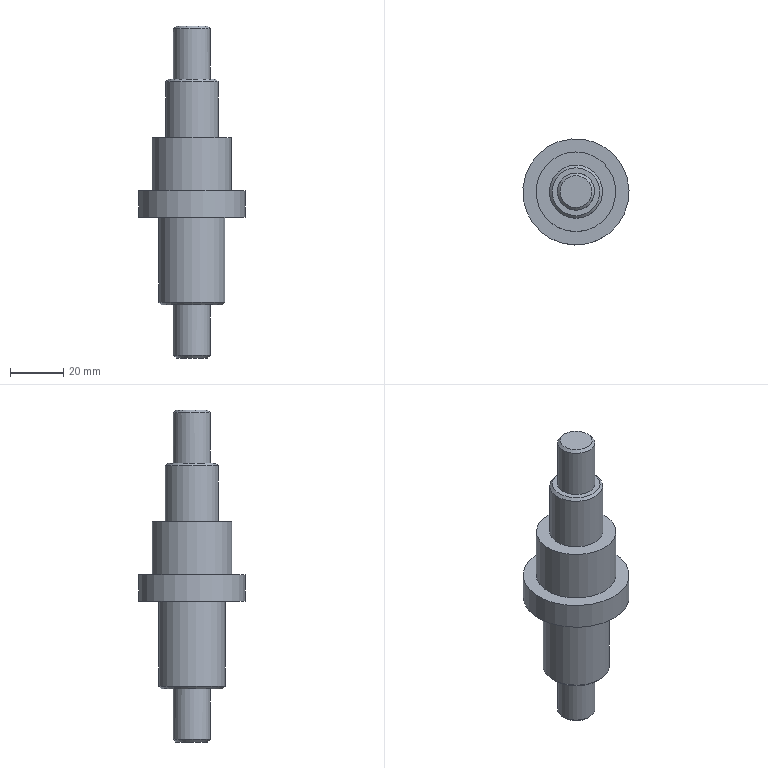Part | STEP file | HL4GZ-1.313.202 (eye-ring mounting shaft) | 1 solid | 17 faces | box 40 x 40 x 125 mm | volume 55861 mm3 | plane 7 | cylinder 6 | cone 4 | commonest cylinder face diameters 14 x2 20 x1 25 x1 30 x1 40 x1
STEP:
#1=CARTESIAN_POINT('',(0.,0.,0.));
#2=DIRECTION('',(0.,0.,1.));
#3=DIRECTION('',(1.,0.,0.));
#4=AXIS2_PLACEMENT_3D('',#1,#2,#3);
#5=CARTESIAN_POINT('',(2574.634,152.537,54.));
#6=VERTEX_POINT('',#5);
#7=CARTESIAN_POINT('',(2570.663,148.04,54.));
#8=DIRECTION('',(0.,0.,-1.));
#9=DIRECTION('',(-0.6618,-0.7497,0.));
#10=AXIS2_PLACEMENT_3D('',#7,#8,#9);
#11=CIRCLE('',#10,6.);
#12=CARTESIAN_POINT('',(2566.03,142.792,54.));
#13=DIRECTION('',(0.,0.,1.));
#14=DIRECTION('',(-0.1489,0.9889,0.));
#15=AXIS2_PLACEMENT_3D('',#12,#13,#14);
#16=PLANE('',#15);
#17=CARTESIAN_POINT('',(0.6428,-0.766));
#18=CARTESIAN_POINT('',(8.604,5.914));
#19=CARTESIAN_POINT('',(10.408,-4.32));
#20=CARTESIAN_POINT('',(12.213,-14.555));
#21=CARTESIAN_POINT('',(2.447,-11.));
#22=CARTESIAN_POINT('',(-7.318,-7.446));
#23=CARTESIAN_POINT('',(0.6428,-0.766));
#24=(BOUNDED_CURVE()B_SPLINE_CURVE(2,(#17,#18,#19,#20,#21,#22,#23),.UNSPECIFIED.,.T.,.F.)B_SPLINE_CURVE_WITH_KNOTS((1,2,2,2,2,1),(-2.094,0.,2.094,4.189,6.283,8.378),.UNSPECIFIED.)CURVE()GEOMETRIC_REPRESENTATION_ITEM()RATIONAL_B_SPLINE_CURVE((1.,0.5,1.,0.5,1.,0.5,1.))REPRESENTATION_ITEM(''));
#25=(GEOMETRIC_REPRESENTATION_CONTEXT(2)PARAMETRIC_REPRESENTATION_CONTEXT()REPRESENTATION_CONTEXT('',''));
#26=DEFINITIONAL_REPRESENTATION('',(#24),#25);
#27=PCURVE('',#16,#26);
#28=CARTESIAN_POINT('',(2570.663,148.04,53.5));
#29=DIRECTION('',(0.,0.,-1.));
#30=DIRECTION('',(-0.6618,-0.7497,0.));
#31=AXIS2_PLACEMENT_3D('',#28,#29,#30);
#32=CONICAL_SURFACE('',#31,6.5,0.7854);
#33=CARTESIAN_POINT('',(0.,-0.5));
#34=DIRECTION('',(1.,0.));
#35=VECTOR('',#34,1.);
#36=LINE('',#33,#35);
#37=(GEOMETRIC_REPRESENTATION_CONTEXT(2)PARAMETRIC_REPRESENTATION_CONTEXT()REPRESENTATION_CONTEXT('',''));
#38=DEFINITIONAL_REPRESENTATION('',(#36),#37);
#39=PCURVE('',#32,#38);
#40=SURFACE_CURVE('',#11,(#27,#39),.PCURVE_S1.);
#41=EDGE_CURVE('',#6,#6,#40,.T.);
#42=ORIENTED_EDGE('',*,*,#41,.F.);
#43=EDGE_LOOP('',(#42));
#44=FACE_BOUND('',#43,.T.);
#45=ADVANCED_FACE('',(#44),#16,.T.);
#46=CARTESIAN_POINT('',(2575.296,153.287,53.));
#47=VERTEX_POINT('',#46);
#48=CARTESIAN_POINT('',(2577.585,149.082,53.));
#49=VERTEX_POINT('',#48);
#50=CARTESIAN_POINT('',(2570.663,148.04,53.));
#51=DIRECTION('',(0.,0.,1.));
#52=DIRECTION('',(-0.6618,-0.7497,0.));
#53=AXIS2_PLACEMENT_3D('',#50,#51,#52);
#54=CIRCLE('',#53,7.);
#55=CARTESIAN_POINT('',(12.566,0.5));
#56=DIRECTION('',(-1.,0.));
#57=VECTOR('',#56,1.);
#58=LINE('',#55,#57);
#59=(GEOMETRIC_REPRESENTATION_CONTEXT(2)PARAMETRIC_REPRESENTATION_CONTEXT()REPRESENTATION_CONTEXT('',''));
#60=DEFINITIONAL_REPRESENTATION('',(#58),#59);
#61=PCURVE('',#32,#60);
#62=CARTESIAN_POINT('',(2570.663,148.04,37.));
#63=DIRECTION('',(0.,0.,-1.));
#64=DIRECTION('',(-0.6618,-0.7497,0.));
#65=AXIS2_PLACEMENT_3D('',#62,#63,#64);
#66=CYLINDRICAL_SURFACE('',#65,7.);
#67=CARTESIAN_POINT('',(12.566,-16.));
#68=DIRECTION('',(-1.,0.));
#69=VECTOR('',#68,1.);
#70=LINE('',#67,#69);
#71=(GEOMETRIC_REPRESENTATION_CONTEXT(2)PARAMETRIC_REPRESENTATION_CONTEXT()REPRESENTATION_CONTEXT('',''));
#72=DEFINITIONAL_REPRESENTATION('',(#70),#71);
#73=PCURVE('',#66,#72);
#74=SURFACE_CURVE('',#54,(#61,#73),.PCURVE_S1.);
#75=EDGE_CURVE('',#47,#49,#74,.T.);
#76=ORIENTED_EDGE('',*,*,#75,.T.);
#77=CARTESIAN_POINT('',(2570.663,148.04,53.));
#78=DIRECTION('',(0.,0.,1.));
#79=DIRECTION('',(-0.6618,-0.7497,0.));
#80=AXIS2_PLACEMENT_3D('',#77,#78,#79);
#81=CIRCLE('',#80,7.);
#82=CARTESIAN_POINT('',(6.283,0.5));
#83=DIRECTION('',(-1.,0.));
#84=VECTOR('',#83,1.);
#85=LINE('',#82,#84);
#86=(GEOMETRIC_REPRESENTATION_CONTEXT(2)PARAMETRIC_REPRESENTATION_CONTEXT()REPRESENTATION_CONTEXT('',''));
#87=DEFINITIONAL_REPRESENTATION('',(#85),#86);
#88=PCURVE('',#32,#87);
#89=CARTESIAN_POINT('',(12.566,-16.));
#90=DIRECTION('',(-1.,0.));
#91=VECTOR('',#90,1.);
#92=LINE('',#89,#91);
#93=(GEOMETRIC_REPRESENTATION_CONTEXT(2)PARAMETRIC_REPRESENTATION_CONTEXT()REPRESENTATION_CONTEXT('',''));
#94=DEFINITIONAL_REPRESENTATION('',(#92),#93);
#95=PCURVE('',#66,#94);
#96=SURFACE_CURVE('',#81,(#88,#95),.PCURVE_S1.);
#97=EDGE_CURVE('',#49,#47,#96,.T.);
#98=ORIENTED_EDGE('',*,*,#97,.T.);
#99=CARTESIAN_POINT('',(2574.634,152.537,54.));
#100=CARTESIAN_POINT('',(2575.296,153.287,53.));
#101=B_SPLINE_CURVE_WITH_KNOTS('',1,(#99,#100),.UNSPECIFIED.,.F.,.F.,(2,2),(-0.7071,0.7071),.PIECEWISE_BEZIER_KNOTS.);
#102=CARTESIAN_POINT('',(3.142,0.));
#103=DIRECTION('',(0.,1.));
#104=VECTOR('',#103,1.);
#105=LINE('',#102,#104);
#106=(GEOMETRIC_REPRESENTATION_CONTEXT(2)PARAMETRIC_REPRESENTATION_CONTEXT()REPRESENTATION_CONTEXT('',''));
#107=DEFINITIONAL_REPRESENTATION('',(#105),#106);
#108=PCURVE('',#32,#107);
#109=CARTESIAN_POINT('',(9.425,0.));
#110=DIRECTION('',(0.,1.));
#111=VECTOR('',#110,1.);
#112=LINE('',#109,#111);
#113=(GEOMETRIC_REPRESENTATION_CONTEXT(2)PARAMETRIC_REPRESENTATION_CONTEXT()REPRESENTATION_CONTEXT('',''));
#114=DEFINITIONAL_REPRESENTATION('',(#112),#113);
#115=PCURVE('',#32,#114);
#116=SEAM_CURVE('',#101,(#108,#115),.PCURVE_S1.);
#117=EDGE_CURVE('',#6,#47,#116,.T.);
#118=ORIENTED_EDGE('',*,*,#117,.F.);
#119=ORIENTED_EDGE('',*,*,#41,.T.);
#120=ORIENTED_EDGE('',*,*,#117,.T.);
#121=EDGE_LOOP('',(#76,#98,#118,#119,#120));
#122=FACE_BOUND('',#121,.T.);
#123=ADVANCED_FACE('',(#122),#32,.T.);
#124=ORIENTED_EDGE('',*,*,#97,.F.);
#125=CARTESIAN_POINT('',(2577.585,149.082,34.));
#126=VERTEX_POINT('',#125);
#127=CARTESIAN_POINT('',(2577.585,149.082,53.));
#128=CARTESIAN_POINT('',(2577.585,149.082,34.));
#129=B_SPLINE_CURVE_WITH_KNOTS('',1,(#127,#128),.UNSPECIFIED.,.F.,.F.,(2,2),(-16.,3.),.PIECEWISE_BEZIER_KNOTS.);
#130=CARTESIAN_POINT('',(10.123,0.));
#131=DIRECTION('',(0.,1.));
#132=VECTOR('',#131,1.);
#133=LINE('',#130,#132);
#134=(GEOMETRIC_REPRESENTATION_CONTEXT(2)PARAMETRIC_REPRESENTATION_CONTEXT()REPRESENTATION_CONTEXT('',''));
#135=DEFINITIONAL_REPRESENTATION('',(#133),#134);
#136=PCURVE('',#66,#135);
#137=CARTESIAN_POINT('',(3.84,0.));
#138=DIRECTION('',(0.,1.));
#139=VECTOR('',#138,1.);
#140=LINE('',#137,#139);
#141=(GEOMETRIC_REPRESENTATION_CONTEXT(2)PARAMETRIC_REPRESENTATION_CONTEXT()REPRESENTATION_CONTEXT('',''));
#142=DEFINITIONAL_REPRESENTATION('',(#140),#141);
#143=PCURVE('',#66,#142);
#144=SEAM_CURVE('',#129,(#136,#143),.PCURVE_S1.);
#145=EDGE_CURVE('',#49,#126,#144,.T.);
#146=ORIENTED_EDGE('',*,*,#145,.T.);
#147=CARTESIAN_POINT('',(2570.663,148.04,34.));
#148=DIRECTION('',(0.,0.,-1.));
#149=DIRECTION('',(-0.9889,-0.1489,0.));
#150=AXIS2_PLACEMENT_3D('',#147,#148,#149);
#151=CIRCLE('',#150,7.);
#152=CARTESIAN_POINT('',(0.6981,3.));
#153=DIRECTION('',(1.,0.));
#154=VECTOR('',#153,1.);
#155=LINE('',#152,#154);
#156=(GEOMETRIC_REPRESENTATION_CONTEXT(2)PARAMETRIC_REPRESENTATION_CONTEXT()REPRESENTATION_CONTEXT('',''));
#157=DEFINITIONAL_REPRESENTATION('',(#155),#156);
#158=PCURVE('',#66,#157);
#159=CARTESIAN_POINT('',(2562.39,138.669,34.));
#160=DIRECTION('',(0.,0.,1.));
#161=DIRECTION('',(-0.1489,0.9889,0.));
#162=AXIS2_PLACEMENT_3D('',#159,#160,#161);
#163=PLANE('',#162);
#164=CARTESIAN_POINT('',(8.035,-2.576));
#165=CARTESIAN_POINT('',(20.159,-2.576));
#166=CARTESIAN_POINT('',(14.097,-13.076));
#167=CARTESIAN_POINT('',(8.035,-23.576));
#168=CARTESIAN_POINT('',(1.973,-13.076));
#169=CARTESIAN_POINT('',(-4.09,-2.576));
#170=CARTESIAN_POINT('',(8.035,-2.576));
#171=(BOUNDED_CURVE()B_SPLINE_CURVE(2,(#164,#165,#166,#167,#168,#169,#170),.UNSPECIFIED.,.T.,.F.)B_SPLINE_CURVE_WITH_KNOTS((1,2,2,2,2,1),(-2.094,0.,2.094,4.189,6.283,8.378),.UNSPECIFIED.)CURVE()GEOMETRIC_REPRESENTATION_ITEM()RATIONAL_B_SPLINE_CURVE((1.,0.5,1.,0.5,1.,0.5,1.))REPRESENTATION_ITEM(''));
#172=(GEOMETRIC_REPRESENTATION_CONTEXT(2)PARAMETRIC_REPRESENTATION_CONTEXT()REPRESENTATION_CONTEXT('',''));
#173=DEFINITIONAL_REPRESENTATION('',(#171),#172);
#174=PCURVE('',#163,#173);
#175=SURFACE_CURVE('',#151,(#158,#174),.PCURVE_S1.);
#176=EDGE_CURVE('',#126,#126,#175,.T.);
#177=ORIENTED_EDGE('',*,*,#176,.F.);
#178=ORIENTED_EDGE('',*,*,#145,.F.);
#179=ORIENTED_EDGE('',*,*,#75,.F.);
#180=EDGE_LOOP('',(#124,#146,#177,#178,#179));
#181=FACE_BOUND('',#180,.T.);
#182=ADVANCED_FACE('',(#181),#66,.T.);
#183=ORIENTED_EDGE('',*,*,#176,.T.);
#184=EDGE_LOOP('',(#183));
#185=FACE_BOUND('',#184,.T.);
#186=CARTESIAN_POINT('',(2576.619,154.786,34.));
#187=VERTEX_POINT('',#186);
#188=CARTESIAN_POINT('',(2570.663,148.04,34.));
#189=DIRECTION('',(0.,0.,-1.));
#190=DIRECTION('',(-0.6618,-0.7497,0.));
#191=AXIS2_PLACEMENT_3D('',#188,#189,#190);
#192=CIRCLE('',#191,9.);
#193=CARTESIAN_POINT('',(2.25,-2.681));
#194=CARTESIAN_POINT('',(14.191,7.339));
#195=CARTESIAN_POINT('',(16.898,-8.013));
#196=CARTESIAN_POINT('',(19.605,-23.364));
#197=CARTESIAN_POINT('',(4.957,-18.033));
#198=CARTESIAN_POINT('',(-9.692,-12.701));
#199=CARTESIAN_POINT('',(2.25,-2.681));
#200=(BOUNDED_CURVE()B_SPLINE_CURVE(2,(#193,#194,#195,#196,#197,#198,#199),.UNSPECIFIED.,.T.,.F.)B_SPLINE_CURVE_WITH_KNOTS((1,2,2,2,2,1),(-2.094,0.,2.094,4.189,6.283,8.378),.UNSPECIFIED.)CURVE()GEOMETRIC_REPRESENTATION_ITEM()RATIONAL_B_SPLINE_CURVE((1.,0.5,1.,0.5,1.,0.5,1.))REPRESENTATION_ITEM(''));
#201=(GEOMETRIC_REPRESENTATION_CONTEXT(2)PARAMETRIC_REPRESENTATION_CONTEXT()REPRESENTATION_CONTEXT('',''));
#202=DEFINITIONAL_REPRESENTATION('',(#200),#201);
#203=PCURVE('',#163,#202);
#204=CARTESIAN_POINT('',(2570.663,148.04,33.5));
#205=DIRECTION('',(0.,0.,-1.));
#206=DIRECTION('',(-0.6618,-0.7497,0.));
#207=AXIS2_PLACEMENT_3D('',#204,#205,#206);
#208=CONICAL_SURFACE('',#207,9.5,0.7854);
#209=CARTESIAN_POINT('',(0.,-0.5));
#210=DIRECTION('',(1.,0.));
#211=VECTOR('',#210,1.);
#212=LINE('',#209,#211);
#213=(GEOMETRIC_REPRESENTATION_CONTEXT(2)PARAMETRIC_REPRESENTATION_CONTEXT()REPRESENTATION_CONTEXT('',''));
#214=DEFINITIONAL_REPRESENTATION('',(#212),#213);
#215=PCURVE('',#208,#214);
#216=SURFACE_CURVE('',#192,(#203,#215),.PCURVE_S1.);
#217=EDGE_CURVE('',#187,#187,#216,.T.);
#218=ORIENTED_EDGE('',*,*,#217,.F.);
#219=EDGE_LOOP('',(#218));
#220=FACE_BOUND('',#219,.T.);
#221=ADVANCED_FACE('',(#185,#220),#163,.T.);
#222=CARTESIAN_POINT('',(2577.281,155.536,33.));
#223=VERTEX_POINT('',#222);
#224=CARTESIAN_POINT('',(2570.663,148.04,33.));
#225=DIRECTION('',(0.,0.,1.));
#226=DIRECTION('',(-0.6618,-0.7497,0.));
#227=AXIS2_PLACEMENT_3D('',#224,#225,#226);
#228=CIRCLE('',#227,10.);
#229=CARTESIAN_POINT('',(12.566,0.5));
#230=DIRECTION('',(-1.,0.));
#231=VECTOR('',#230,1.);
#232=LINE('',#229,#231);
#233=(GEOMETRIC_REPRESENTATION_CONTEXT(2)PARAMETRIC_REPRESENTATION_CONTEXT()REPRESENTATION_CONTEXT('',''));
#234=DEFINITIONAL_REPRESENTATION('',(#232),#233);
#235=PCURVE('',#208,#234);
#236=CARTESIAN_POINT('',(2570.663,148.04,17.));
#237=DIRECTION('',(0.,0.,-1.));
#238=DIRECTION('',(-0.6618,-0.7497,0.));
#239=AXIS2_PLACEMENT_3D('',#236,#237,#238);
#240=CYLINDRICAL_SURFACE('',#239,10.);
#241=CARTESIAN_POINT('',(12.566,-16.));
#242=DIRECTION('',(-1.,0.));
#243=VECTOR('',#242,1.);
#244=LINE('',#241,#243);
#245=(GEOMETRIC_REPRESENTATION_CONTEXT(2)PARAMETRIC_REPRESENTATION_CONTEXT()REPRESENTATION_CONTEXT('',''));
#246=DEFINITIONAL_REPRESENTATION('',(#244),#245);
#247=PCURVE('',#240,#246);
#248=SURFACE_CURVE('',#228,(#235,#247),.PCURVE_S1.);
#249=EDGE_CURVE('',#223,#223,#248,.T.);
#250=ORIENTED_EDGE('',*,*,#249,.T.);
#251=CARTESIAN_POINT('',(2576.619,154.786,34.));
#252=CARTESIAN_POINT('',(2577.281,155.536,33.));
#253=B_SPLINE_CURVE_WITH_KNOTS('',1,(#251,#252),.UNSPECIFIED.,.F.,.F.,(2,2),(-0.7071,0.7071),.PIECEWISE_BEZIER_KNOTS.);
#254=CARTESIAN_POINT('',(3.142,0.));
#255=DIRECTION('',(0.,1.));
#256=VECTOR('',#255,1.);
#257=LINE('',#254,#256);
#258=(GEOMETRIC_REPRESENTATION_CONTEXT(2)PARAMETRIC_REPRESENTATION_CONTEXT()REPRESENTATION_CONTEXT('',''));
#259=DEFINITIONAL_REPRESENTATION('',(#257),#258);
#260=PCURVE('',#208,#259);
#261=CARTESIAN_POINT('',(9.425,0.));
#262=DIRECTION('',(0.,1.));
#263=VECTOR('',#262,1.);
#264=LINE('',#261,#263);
#265=(GEOMETRIC_REPRESENTATION_CONTEXT(2)PARAMETRIC_REPRESENTATION_CONTEXT()REPRESENTATION_CONTEXT('',''));
#266=DEFINITIONAL_REPRESENTATION('',(#264),#265);
#267=PCURVE('',#208,#266);
#268=SEAM_CURVE('',#253,(#260,#267),.PCURVE_S1.);
#269=EDGE_CURVE('',#187,#223,#268,.T.);
#270=ORIENTED_EDGE('',*,*,#269,.F.);
#271=ORIENTED_EDGE('',*,*,#217,.T.);
#272=ORIENTED_EDGE('',*,*,#269,.T.);
#273=EDGE_LOOP('',(#250,#270,#271,#272));
#274=FACE_BOUND('',#273,.T.);
#275=ADVANCED_FACE('',(#274),#208,.T.);
#276=ORIENTED_EDGE('',*,*,#249,.F.);
#277=CARTESIAN_POINT('',(2577.281,155.536,12.));
#278=VERTEX_POINT('',#277);
#279=CARTESIAN_POINT('',(2577.281,155.536,33.));
#280=CARTESIAN_POINT('',(2577.281,155.536,12.));
#281=B_SPLINE_CURVE_WITH_KNOTS('',1,(#279,#280),.UNSPECIFIED.,.F.,.F.,(2,2),(-16.,5.),.PIECEWISE_BEZIER_KNOTS.);
#282=CARTESIAN_POINT('',(9.425,0.));
#283=DIRECTION('',(0.,1.));
#284=VECTOR('',#283,1.);
#285=LINE('',#282,#284);
#286=(GEOMETRIC_REPRESENTATION_CONTEXT(2)PARAMETRIC_REPRESENTATION_CONTEXT()REPRESENTATION_CONTEXT('',''));
#287=DEFINITIONAL_REPRESENTATION('',(#285),#286);
#288=PCURVE('',#240,#287);
#289=CARTESIAN_POINT('',(3.142,0.));
#290=DIRECTION('',(0.,1.));
#291=VECTOR('',#290,1.);
#292=LINE('',#289,#291);
#293=(GEOMETRIC_REPRESENTATION_CONTEXT(2)PARAMETRIC_REPRESENTATION_CONTEXT()REPRESENTATION_CONTEXT('',''));
#294=DEFINITIONAL_REPRESENTATION('',(#292),#293);
#295=PCURVE('',#240,#294);
#296=SEAM_CURVE('',#281,(#288,#295),.PCURVE_S1.);
#297=EDGE_CURVE('',#223,#278,#296,.T.);
#298=ORIENTED_EDGE('',*,*,#297,.T.);
#299=CARTESIAN_POINT('',(2570.663,148.04,12.));
#300=DIRECTION('',(0.,0.,-1.));
#301=DIRECTION('',(-0.6618,-0.7497,0.));
#302=AXIS2_PLACEMENT_3D('',#299,#300,#301);
#303=CIRCLE('',#302,10.);
#304=CARTESIAN_POINT('',(0.,5.));
#305=DIRECTION('',(1.,0.));
#306=VECTOR('',#305,1.);
#307=LINE('',#304,#306);
#308=(GEOMETRIC_REPRESENTATION_CONTEXT(2)PARAMETRIC_REPRESENTATION_CONTEXT()REPRESENTATION_CONTEXT('',''));
#309=DEFINITIONAL_REPRESENTATION('',(#307),#308);
#310=PCURVE('',#240,#309);
#311=CARTESIAN_POINT('',(2560.736,136.795,12.));
#312=DIRECTION('',(0.,0.,1.));
#313=DIRECTION('',(-0.1489,0.9889,0.));
#314=AXIS2_PLACEMENT_3D('',#311,#312,#313);
#315=PLANE('',#314);
#316=CARTESIAN_POINT('',(3.214,-3.83));
#317=CARTESIAN_POINT('',(16.482,7.303));
#318=CARTESIAN_POINT('',(19.49,-9.754));
#319=CARTESIAN_POINT('',(22.498,-26.812));
#320=CARTESIAN_POINT('',(6.222,-20.888));
#321=CARTESIAN_POINT('',(-10.054,-14.964));
#322=CARTESIAN_POINT('',(3.214,-3.83));
#323=(BOUNDED_CURVE()B_SPLINE_CURVE(2,(#316,#317,#318,#319,#320,#321,#322),.UNSPECIFIED.,.T.,.F.)B_SPLINE_CURVE_WITH_KNOTS((1,2,2,2,2,1),(-2.094,0.,2.094,4.189,6.283,8.378),.UNSPECIFIED.)CURVE()GEOMETRIC_REPRESENTATION_ITEM()RATIONAL_B_SPLINE_CURVE((1.,0.5,1.,0.5,1.,0.5,1.))REPRESENTATION_ITEM(''));
#324=(GEOMETRIC_REPRESENTATION_CONTEXT(2)PARAMETRIC_REPRESENTATION_CONTEXT()REPRESENTATION_CONTEXT('',''));
#325=DEFINITIONAL_REPRESENTATION('',(#323),#324);
#326=PCURVE('',#315,#325);
#327=SURFACE_CURVE('',#303,(#310,#326),.PCURVE_S1.);
#328=EDGE_CURVE('',#278,#278,#327,.T.);
#329=ORIENTED_EDGE('',*,*,#328,.F.);
#330=ORIENTED_EDGE('',*,*,#297,.F.);
#331=EDGE_LOOP('',(#276,#298,#329,#330));
#332=FACE_BOUND('',#331,.T.);
#333=ADVANCED_FACE('',(#332),#240,.T.);
#334=ORIENTED_EDGE('',*,*,#328,.T.);
#335=EDGE_LOOP('',(#334));
#336=FACE_BOUND('',#335,.T.);
#337=CARTESIAN_POINT('',(2580.59,159.284,12.));
#338=VERTEX_POINT('',#337);
#339=CARTESIAN_POINT('',(2560.736,136.795,12.));
#340=VERTEX_POINT('',#339);
#341=CARTESIAN_POINT('',(2570.663,148.04,12.));
#342=DIRECTION('',(0.,0.,-1.));
#343=DIRECTION('',(-0.6618,-0.7497,0.));
#344=AXIS2_PLACEMENT_3D('',#341,#342,#343);
#345=CIRCLE('',#344,15.);
#346=CARTESIAN_POINT('',(0.,0.));
#347=CARTESIAN_POINT('',(19.902,16.7));
#348=CARTESIAN_POINT('',(24.414,-8.886));
#349=CARTESIAN_POINT('',(28.925,-34.472));
#350=CARTESIAN_POINT('',(4.512,-25.586));
#351=CARTESIAN_POINT('',(-19.902,-16.7));
#352=CARTESIAN_POINT('',(0.,0.));
#353=(BOUNDED_CURVE()B_SPLINE_CURVE(2,(#346,#347,#348,#349,#350,#351,#352),.UNSPECIFIED.,.T.,.F.)B_SPLINE_CURVE_WITH_KNOTS((1,2,2,2,2,1),(-2.094,0.,2.094,4.189,6.283,8.378),.UNSPECIFIED.)CURVE()GEOMETRIC_REPRESENTATION_ITEM()RATIONAL_B_SPLINE_CURVE((1.,0.5,1.,0.5,1.,0.5,1.))REPRESENTATION_ITEM(''));
#354=(GEOMETRIC_REPRESENTATION_CONTEXT(2)PARAMETRIC_REPRESENTATION_CONTEXT()REPRESENTATION_CONTEXT('',''));
#355=DEFINITIONAL_REPRESENTATION('',(#353),#354);
#356=PCURVE('',#315,#355);
#357=CARTESIAN_POINT('',(2570.663,148.04,-0.5));
#358=DIRECTION('',(0.,0.,-1.));
#359=DIRECTION('',(-0.6618,-0.7497,0.));
#360=AXIS2_PLACEMENT_3D('',#357,#358,#359);
#361=CYLINDRICAL_SURFACE('',#360,15.);
#362=CARTESIAN_POINT('',(0.,-12.5));
#363=DIRECTION('',(1.,0.));
#364=VECTOR('',#363,1.);
#365=LINE('',#362,#364);
#366=(GEOMETRIC_REPRESENTATION_CONTEXT(2)PARAMETRIC_REPRESENTATION_CONTEXT()REPRESENTATION_CONTEXT('',''));
#367=DEFINITIONAL_REPRESENTATION('',(#365),#366);
#368=PCURVE('',#361,#367);
#369=SURFACE_CURVE('',#345,(#356,#368),.PCURVE_S1.);
#370=EDGE_CURVE('',#338,#340,#369,.T.);
#371=ORIENTED_EDGE('',*,*,#370,.F.);
#372=CARTESIAN_POINT('',(2570.663,148.04,12.));
#373=DIRECTION('',(0.,0.,-1.));
#374=DIRECTION('',(-0.6618,-0.7497,0.));
#375=AXIS2_PLACEMENT_3D('',#372,#373,#374);
#376=CIRCLE('',#375,15.);
#377=CARTESIAN_POINT('',(0.,0.));
#378=CARTESIAN_POINT('',(19.902,16.7));
#379=CARTESIAN_POINT('',(24.414,-8.886));
#380=CARTESIAN_POINT('',(28.925,-34.472));
#381=CARTESIAN_POINT('',(4.512,-25.586));
#382=CARTESIAN_POINT('',(-19.902,-16.7));
#383=CARTESIAN_POINT('',(0.,0.));
#384=(BOUNDED_CURVE()B_SPLINE_CURVE(2,(#377,#378,#379,#380,#381,#382,#383),.UNSPECIFIED.,.T.,.F.)B_SPLINE_CURVE_WITH_KNOTS((1,2,2,2,2,1),(-2.094,0.,2.094,4.189,6.283,8.378),.UNSPECIFIED.)CURVE()GEOMETRIC_REPRESENTATION_ITEM()RATIONAL_B_SPLINE_CURVE((1.,0.5,1.,0.5,1.,0.5,1.))REPRESENTATION_ITEM(''));
#385=(GEOMETRIC_REPRESENTATION_CONTEXT(2)PARAMETRIC_REPRESENTATION_CONTEXT()REPRESENTATION_CONTEXT('',''));
#386=DEFINITIONAL_REPRESENTATION('',(#384),#385);
#387=PCURVE('',#315,#386);
#388=CARTESIAN_POINT('',(-6.283,-12.5));
#389=DIRECTION('',(1.,0.));
#390=VECTOR('',#389,1.);
#391=LINE('',#388,#390);
#392=(GEOMETRIC_REPRESENTATION_CONTEXT(2)PARAMETRIC_REPRESENTATION_CONTEXT()REPRESENTATION_CONTEXT('',''));
#393=DEFINITIONAL_REPRESENTATION('',(#391),#392);
#394=PCURVE('',#361,#393);
#395=SURFACE_CURVE('',#376,(#387,#394),.PCURVE_S1.);
#396=EDGE_CURVE('',#340,#338,#395,.T.);
#397=ORIENTED_EDGE('',*,*,#396,.F.);
#398=EDGE_LOOP('',(#371,#397));
#399=FACE_BOUND('',#398,.T.);
#400=ADVANCED_FACE('',(#336,#399),#315,.T.);
#401=CARTESIAN_POINT('',(2560.736,136.795,-8.));
#402=VERTEX_POINT('',#401);
#403=CARTESIAN_POINT('',(2570.663,148.04,-8.));
#404=DIRECTION('',(0.,0.,-1.));
#405=DIRECTION('',(0.9889,0.1489,0.));
#406=AXIS2_PLACEMENT_3D('',#403,#404,#405);
#407=CIRCLE('',#406,15.);
#408=CARTESIAN_POINT('',(-2.443,7.5));
#409=DIRECTION('',(1.,0.));
#410=VECTOR('',#409,1.);
#411=LINE('',#408,#410);
#412=(GEOMETRIC_REPRESENTATION_CONTEXT(2)PARAMETRIC_REPRESENTATION_CONTEXT()REPRESENTATION_CONTEXT('',''));
#413=DEFINITIONAL_REPRESENTATION('',(#411),#412);
#414=PCURVE('',#361,#413);
#415=CARTESIAN_POINT('',(2557.427,133.046,-8.));
#416=DIRECTION('',(0.,0.,1.));
#417=DIRECTION('',(-0.1489,0.9889,0.));
#418=AXIS2_PLACEMENT_3D('',#415,#416,#417);
#419=PLANE('',#418);
#420=CARTESIAN_POINT('',(12.856,-30.321));
#421=CARTESIAN_POINT('',(-13.125,-30.321));
#422=CARTESIAN_POINT('',(-0.1346,-7.821));
#423=CARTESIAN_POINT('',(12.856,14.679));
#424=CARTESIAN_POINT('',(25.846,-7.821));
#425=CARTESIAN_POINT('',(38.837,-30.321));
#426=CARTESIAN_POINT('',(12.856,-30.321));
#427=(BOUNDED_CURVE()B_SPLINE_CURVE(2,(#420,#421,#422,#423,#424,#425,#426),.UNSPECIFIED.,.T.,.F.)B_SPLINE_CURVE_WITH_KNOTS((1,2,2,2,2,1),(-2.094,0.,2.094,4.189,6.283,8.378),.UNSPECIFIED.)CURVE()GEOMETRIC_REPRESENTATION_ITEM()RATIONAL_B_SPLINE_CURVE((1.,0.5,1.,0.5,1.,0.5,1.))REPRESENTATION_ITEM(''));
#428=(GEOMETRIC_REPRESENTATION_CONTEXT(2)PARAMETRIC_REPRESENTATION_CONTEXT()REPRESENTATION_CONTEXT('',''));
#429=DEFINITIONAL_REPRESENTATION('',(#427),#428);
#430=PCURVE('',#419,#429);
#431=SURFACE_CURVE('',#407,(#414,#430),.PCURVE_S1.);
#432=EDGE_CURVE('',#402,#402,#431,.T.);
#433=ORIENTED_EDGE('',*,*,#432,.F.);
#434=CARTESIAN_POINT('',(2560.736,136.795,12.));
#435=CARTESIAN_POINT('',(2560.736,136.795,-8.));
#436=B_SPLINE_CURVE_WITH_KNOTS('',1,(#434,#435),.UNSPECIFIED.,.F.,.F.,(2,2),(-12.5,7.5),.PIECEWISE_BEZIER_KNOTS.);
#437=CARTESIAN_POINT('',(0.,0.));
#438=DIRECTION('',(0.,1.));
#439=VECTOR('',#438,1.);
#440=LINE('',#437,#439);
#441=(GEOMETRIC_REPRESENTATION_CONTEXT(2)PARAMETRIC_REPRESENTATION_CONTEXT()REPRESENTATION_CONTEXT('',''));
#442=DEFINITIONAL_REPRESENTATION('',(#440),#441);
#443=PCURVE('',#361,#442);
#444=CARTESIAN_POINT('',(6.283,0.));
#445=DIRECTION('',(0.,1.));
#446=VECTOR('',#445,1.);
#447=LINE('',#444,#446);
#448=(GEOMETRIC_REPRESENTATION_CONTEXT(2)PARAMETRIC_REPRESENTATION_CONTEXT()REPRESENTATION_CONTEXT('',''));
#449=DEFINITIONAL_REPRESENTATION('',(#447),#448);
#450=PCURVE('',#361,#449);
#451=SEAM_CURVE('',#436,(#443,#450),.PCURVE_S1.);
#452=EDGE_CURVE('',#340,#402,#451,.T.);
#453=ORIENTED_EDGE('',*,*,#452,.F.);
#454=ORIENTED_EDGE('',*,*,#396,.T.);
#455=ORIENTED_EDGE('',*,*,#370,.T.);
#456=ORIENTED_EDGE('',*,*,#452,.T.);
#457=EDGE_LOOP('',(#433,#453,#454,#455,#456));
#458=FACE_BOUND('',#457,.T.);
#459=ADVANCED_FACE('',(#458),#361,.T.);
#460=ORIENTED_EDGE('',*,*,#432,.T.);
#461=EDGE_LOOP('',(#460));
#462=FACE_BOUND('',#461,.T.);
#463=CARTESIAN_POINT('',(2557.427,133.046,-8.));
#464=VERTEX_POINT('',#463);
#465=CARTESIAN_POINT('',(2570.663,148.04,-8.));
#466=DIRECTION('',(0.,0.,-1.));
#467=DIRECTION('',(0.9889,0.1489,0.));
#468=AXIS2_PLACEMENT_3D('',#465,#466,#467);
#469=CIRCLE('',#468,20.);
#470=CARTESIAN_POINT('',(12.856,-35.321));
#471=CARTESIAN_POINT('',(-21.785,-35.321));
#472=CARTESIAN_POINT('',(-4.465,-5.321));
#473=CARTESIAN_POINT('',(12.856,24.679));
#474=CARTESIAN_POINT('',(30.176,-5.321));
#475=CARTESIAN_POINT('',(47.497,-35.321));
#476=CARTESIAN_POINT('',(12.856,-35.321));
#477=(BOUNDED_CURVE()B_SPLINE_CURVE(2,(#470,#471,#472,#473,#474,#475,#476),.UNSPECIFIED.,.T.,.F.)B_SPLINE_CURVE_WITH_KNOTS((1,2,2,2,2,1),(-2.094,0.,2.094,4.189,6.283,8.378),.UNSPECIFIED.)CURVE()GEOMETRIC_REPRESENTATION_ITEM()RATIONAL_B_SPLINE_CURVE((1.,0.5,1.,0.5,1.,0.5,1.))REPRESENTATION_ITEM(''));
#478=(GEOMETRIC_REPRESENTATION_CONTEXT(2)PARAMETRIC_REPRESENTATION_CONTEXT()REPRESENTATION_CONTEXT('',''));
#479=DEFINITIONAL_REPRESENTATION('',(#477),#478);
#480=PCURVE('',#419,#479);
#481=CARTESIAN_POINT('',(2570.663,148.04,-15.5));
#482=DIRECTION('',(0.,0.,-1.));
#483=DIRECTION('',(-0.6618,-0.7497,0.));
#484=AXIS2_PLACEMENT_3D('',#481,#482,#483);
#485=CYLINDRICAL_SURFACE('',#484,20.);
#486=CARTESIAN_POINT('',(-2.443,-7.5));
#487=DIRECTION('',(1.,0.));
#488=VECTOR('',#487,1.);
#489=LINE('',#486,#488);
#490=(GEOMETRIC_REPRESENTATION_CONTEXT(2)PARAMETRIC_REPRESENTATION_CONTEXT()REPRESENTATION_CONTEXT('',''));
#491=DEFINITIONAL_REPRESENTATION('',(#489),#490);
#492=PCURVE('',#485,#491);
#493=SURFACE_CURVE('',#469,(#480,#492),.PCURVE_S1.);
#494=EDGE_CURVE('',#464,#464,#493,.T.);
#495=ORIENTED_EDGE('',*,*,#494,.F.);
#496=EDGE_LOOP('',(#495));
#497=FACE_BOUND('',#496,.T.);
#498=ADVANCED_FACE('',(#462,#497),#419,.T.);
#499=ORIENTED_EDGE('',*,*,#494,.T.);
#500=CARTESIAN_POINT('',(2557.427,133.046,-18.));
#501=VERTEX_POINT('',#500);
#502=CARTESIAN_POINT('',(2557.427,133.046,-8.));
#503=CARTESIAN_POINT('',(2557.427,133.046,-18.));
#504=B_SPLINE_CURVE_WITH_KNOTS('',1,(#502,#503),.UNSPECIFIED.,.F.,.F.,(2,2),(-7.5,2.5),.PIECEWISE_BEZIER_KNOTS.);
#505=CARTESIAN_POINT('',(6.283,0.));
#506=DIRECTION('',(0.,1.));
#507=VECTOR('',#506,1.);
#508=LINE('',#505,#507);
#509=(GEOMETRIC_REPRESENTATION_CONTEXT(2)PARAMETRIC_REPRESENTATION_CONTEXT()REPRESENTATION_CONTEXT('',''));
#510=DEFINITIONAL_REPRESENTATION('',(#508),#509);
#511=PCURVE('',#485,#510);
#512=CARTESIAN_POINT('',(0.,0.));
#513=DIRECTION('',(0.,1.));
#514=VECTOR('',#513,1.);
#515=LINE('',#512,#514);
#516=(GEOMETRIC_REPRESENTATION_CONTEXT(2)PARAMETRIC_REPRESENTATION_CONTEXT()REPRESENTATION_CONTEXT('',''));
#517=DEFINITIONAL_REPRESENTATION('',(#515),#516);
#518=PCURVE('',#485,#517);
#519=SEAM_CURVE('',#504,(#511,#518),.PCURVE_S1.);
#520=EDGE_CURVE('',#464,#501,#519,.T.);
#521=ORIENTED_EDGE('',*,*,#520,.T.);
#522=CARTESIAN_POINT('',(2570.663,148.04,-18.));
#523=DIRECTION('',(0.,0.,-1.));
#524=DIRECTION('',(0.9889,0.1489,0.));
#525=AXIS2_PLACEMENT_3D('',#522,#523,#524);
#526=CIRCLE('',#525,20.);
#527=CARTESIAN_POINT('',(-2.443,2.5));
#528=DIRECTION('',(1.,0.));
#529=VECTOR('',#528,1.);
#530=LINE('',#527,#529);
#531=(GEOMETRIC_REPRESENTATION_CONTEXT(2)PARAMETRIC_REPRESENTATION_CONTEXT()REPRESENTATION_CONTEXT('',''));
#532=DEFINITIONAL_REPRESENTATION('',(#530),#531);
#533=PCURVE('',#485,#532);
#534=CARTESIAN_POINT('',(2562.39,138.669,-18.));
#535=DIRECTION('',(0.,0.,-1.));
#536=DIRECTION('',(0.1489,-0.9889,0.));
#537=AXIS2_PLACEMENT_3D('',#534,#535,#536);
#538=PLANE('',#537);
#539=CARTESIAN_POINT('',(-8.035,-9.576));
#540=DIRECTION('',(0.,-1.));
#541=AXIS2_PLACEMENT_2D('',#539,#540);
#542=CIRCLE('',#541,20.);
#543=(GEOMETRIC_REPRESENTATION_CONTEXT(2)PARAMETRIC_REPRESENTATION_CONTEXT()REPRESENTATION_CONTEXT('',''));
#544=DEFINITIONAL_REPRESENTATION('',(#542),#543);
#545=PCURVE('',#538,#544);
#546=SURFACE_CURVE('',#526,(#533,#545),.PCURVE_S1.);
#547=EDGE_CURVE('',#501,#501,#546,.T.);
#548=ORIENTED_EDGE('',*,*,#547,.F.);
#549=ORIENTED_EDGE('',*,*,#520,.F.);
#550=EDGE_LOOP('',(#499,#521,#548,#549));
#551=FACE_BOUND('',#550,.T.);
#552=ADVANCED_FACE('',(#551),#485,.T.);
#553=CARTESIAN_POINT('',(2562.39,138.669,-18.));
#554=VERTEX_POINT('',#553);
#555=CARTESIAN_POINT('',(2570.663,148.04,-18.));
#556=DIRECTION('',(0.,0.,-1.));
#557=DIRECTION('',(0.9889,0.1489,0.));
#558=AXIS2_PLACEMENT_3D('',#555,#556,#557);
#559=CIRCLE('',#558,12.5);
#560=CARTESIAN_POINT('',(-8.035,-9.576));
#561=DIRECTION('',(0.,-1.));
#562=AXIS2_PLACEMENT_2D('',#560,#561);
#563=CIRCLE('',#562,12.5);
#564=(GEOMETRIC_REPRESENTATION_CONTEXT(2)PARAMETRIC_REPRESENTATION_CONTEXT()REPRESENTATION_CONTEXT('',''));
#565=DEFINITIONAL_REPRESENTATION('',(#563),#564);
#566=PCURVE('',#538,#565);
#567=CARTESIAN_POINT('',(2570.663,148.04,-32.));
#568=DIRECTION('',(0.,0.,-1.));
#569=DIRECTION('',(-0.6618,-0.7497,0.));
#570=AXIS2_PLACEMENT_3D('',#567,#568,#569);
#571=CYLINDRICAL_SURFACE('',#570,12.5);
#572=CARTESIAN_POINT('',(-2.443,-14.));
#573=DIRECTION('',(1.,0.));
#574=VECTOR('',#573,1.);
#575=LINE('',#572,#574);
#576=(GEOMETRIC_REPRESENTATION_CONTEXT(2)PARAMETRIC_REPRESENTATION_CONTEXT()REPRESENTATION_CONTEXT('',''));
#577=DEFINITIONAL_REPRESENTATION('',(#575),#576);
#578=PCURVE('',#571,#577);
#579=SURFACE_CURVE('',#559,(#566,#578),.PCURVE_S1.);
#580=EDGE_CURVE('',#554,#554,#579,.T.);
#581=ORIENTED_EDGE('',*,*,#580,.F.);
#582=EDGE_LOOP('',(#581));
#583=FACE_BOUND('',#582,.T.);
#584=ORIENTED_EDGE('',*,*,#547,.T.);
#585=EDGE_LOOP('',(#584));
#586=FACE_BOUND('',#585,.T.);
#587=ADVANCED_FACE('',(#583,#586),#538,.T.);
#588=ORIENTED_EDGE('',*,*,#580,.T.);
#589=CARTESIAN_POINT('',(2562.39,138.669,-50.));
#590=VERTEX_POINT('',#589);
#591=CARTESIAN_POINT('',(2562.39,138.669,-18.));
#592=CARTESIAN_POINT('',(2562.39,138.669,-50.));
#593=B_SPLINE_CURVE_WITH_KNOTS('',1,(#591,#592),.UNSPECIFIED.,.F.,.F.,(2,2),(-14.,18.),.PIECEWISE_BEZIER_KNOTS.);
#594=CARTESIAN_POINT('',(6.283,0.));
#595=DIRECTION('',(0.,1.));
#596=VECTOR('',#595,1.);
#597=LINE('',#594,#596);
#598=(GEOMETRIC_REPRESENTATION_CONTEXT(2)PARAMETRIC_REPRESENTATION_CONTEXT()REPRESENTATION_CONTEXT('',''));
#599=DEFINITIONAL_REPRESENTATION('',(#597),#598);
#600=PCURVE('',#571,#599);
#601=CARTESIAN_POINT('',(0.,0.));
#602=DIRECTION('',(0.,1.));
#603=VECTOR('',#602,1.);
#604=LINE('',#601,#603);
#605=(GEOMETRIC_REPRESENTATION_CONTEXT(2)PARAMETRIC_REPRESENTATION_CONTEXT()REPRESENTATION_CONTEXT('',''));
#606=DEFINITIONAL_REPRESENTATION('',(#604),#605);
#607=PCURVE('',#571,#606);
#608=SEAM_CURVE('',#593,(#600,#607),.PCURVE_S1.);
#609=EDGE_CURVE('',#554,#590,#608,.T.);
#610=ORIENTED_EDGE('',*,*,#609,.T.);
#611=CARTESIAN_POINT('',(2570.663,148.04,-50.));
#612=DIRECTION('',(0.,0.,-1.));
#613=DIRECTION('',(0.6618,0.7497,0.));
#614=AXIS2_PLACEMENT_3D('',#611,#612,#613);
#615=CIRCLE('',#614,12.5);
#616=CARTESIAN_POINT('',(-3.142,18.));
#617=DIRECTION('',(1.,0.));
#618=VECTOR('',#617,1.);
#619=LINE('',#616,#618);
#620=(GEOMETRIC_REPRESENTATION_CONTEXT(2)PARAMETRIC_REPRESENTATION_CONTEXT()REPRESENTATION_CONTEXT('',''));
#621=DEFINITIONAL_REPRESENTATION('',(#619),#620);
#622=PCURVE('',#571,#621);
#623=CARTESIAN_POINT('',(2570.663,148.04,-50.5));
#624=DIRECTION('',(0.,0.,1.));
#625=DIRECTION('',(0.6618,0.7497,0.));
#626=AXIS2_PLACEMENT_3D('',#623,#624,#625);
#627=CONICAL_SURFACE('',#626,12.,0.7854);
#628=CARTESIAN_POINT('',(12.566,0.5));
#629=DIRECTION('',(-1.,0.));
#630=VECTOR('',#629,1.);
#631=LINE('',#628,#630);
#632=(GEOMETRIC_REPRESENTATION_CONTEXT(2)PARAMETRIC_REPRESENTATION_CONTEXT()REPRESENTATION_CONTEXT('',''));
#633=DEFINITIONAL_REPRESENTATION('',(#631),#632);
#634=PCURVE('',#627,#633);
#635=SURFACE_CURVE('',#615,(#622,#634),.PCURVE_S1.);
#636=EDGE_CURVE('',#590,#590,#635,.T.);
#637=ORIENTED_EDGE('',*,*,#636,.F.);
#638=ORIENTED_EDGE('',*,*,#609,.F.);
#639=EDGE_LOOP('',(#588,#610,#637,#638));
#640=FACE_BOUND('',#639,.T.);
#641=ADVANCED_FACE('',(#640),#571,.T.);
#642=CARTESIAN_POINT('',(2566.692,143.542,-71.));
#643=VERTEX_POINT('',#642);
#644=CARTESIAN_POINT('',(2570.663,148.04,-71.));
#645=DIRECTION('',(0.,0.,1.));
#646=DIRECTION('',(0.6618,0.7497,0.));
#647=AXIS2_PLACEMENT_3D('',#644,#645,#646);
#648=CIRCLE('',#647,6.);
#649=CARTESIAN_POINT('',(2570.663,148.04,-71.));
#650=DIRECTION('',(0.,0.,-1.));
#651=DIRECTION('',(0.1489,-0.9889,0.));
#652=AXIS2_PLACEMENT_3D('',#649,#650,#651);
#653=PLANE('',#652);
#654=CARTESIAN_POINT('',(-3.857,-4.596));
#655=CARTESIAN_POINT('',(-11.818,2.084));
#656=CARTESIAN_POINT('',(-2.052,5.638));
#657=CARTESIAN_POINT('',(7.713,9.193));
#658=CARTESIAN_POINT('',(5.909,-1.042));
#659=CARTESIAN_POINT('',(4.104,-11.276));
#660=CARTESIAN_POINT('',(-3.857,-4.596));
#661=(BOUNDED_CURVE()B_SPLINE_CURVE(2,(#654,#655,#656,#657,#658,#659,#660),.UNSPECIFIED.,.T.,.F.)B_SPLINE_CURVE_WITH_KNOTS((1,2,2,2,2,1),(-2.094,0.,2.094,4.189,6.283,8.378),.UNSPECIFIED.)CURVE()GEOMETRIC_REPRESENTATION_ITEM()RATIONAL_B_SPLINE_CURVE((1.,0.5,1.,0.5,1.,0.5,1.))REPRESENTATION_ITEM(''));
#662=(GEOMETRIC_REPRESENTATION_CONTEXT(2)PARAMETRIC_REPRESENTATION_CONTEXT()REPRESENTATION_CONTEXT('',''));
#663=DEFINITIONAL_REPRESENTATION('',(#661),#662);
#664=PCURVE('',#653,#663);
#665=CARTESIAN_POINT('',(2570.663,148.04,-70.5));
#666=DIRECTION('',(0.,0.,1.));
#667=DIRECTION('',(0.6618,0.7497,0.));
#668=AXIS2_PLACEMENT_3D('',#665,#666,#667);
#669=CONICAL_SURFACE('',#668,6.5,0.7854);
#670=CARTESIAN_POINT('',(0.,-0.5));
#671=DIRECTION('',(1.,0.));
#672=VECTOR('',#671,1.);
#673=LINE('',#670,#672);
#674=(GEOMETRIC_REPRESENTATION_CONTEXT(2)PARAMETRIC_REPRESENTATION_CONTEXT()REPRESENTATION_CONTEXT('',''));
#675=DEFINITIONAL_REPRESENTATION('',(#673),#674);
#676=PCURVE('',#669,#675);
#677=SURFACE_CURVE('',#648,(#664,#676),.PCURVE_S1.);
#678=EDGE_CURVE('',#643,#643,#677,.T.);
#679=ORIENTED_EDGE('',*,*,#678,.F.);
#680=EDGE_LOOP('',(#679));
#681=FACE_BOUND('',#680,.T.);
#682=ADVANCED_FACE('',(#681),#653,.T.);
#683=ORIENTED_EDGE('',*,*,#678,.T.);
#684=CARTESIAN_POINT('',(2566.03,142.792,-70.));
#685=VERTEX_POINT('',#684);
#686=CARTESIAN_POINT('',(2566.692,143.542,-71.));
#687=CARTESIAN_POINT('',(2566.03,142.792,-70.));
#688=B_SPLINE_CURVE_WITH_KNOTS('',1,(#686,#687),.UNSPECIFIED.,.F.,.F.,(2,2),(-0.7071,0.7071),.PIECEWISE_BEZIER_KNOTS.);
#689=CARTESIAN_POINT('',(9.425,0.));
#690=DIRECTION('',(0.,1.));
#691=VECTOR('',#690,1.);
#692=LINE('',#689,#691);
#693=(GEOMETRIC_REPRESENTATION_CONTEXT(2)PARAMETRIC_REPRESENTATION_CONTEXT()REPRESENTATION_CONTEXT('',''));
#694=DEFINITIONAL_REPRESENTATION('',(#692),#693);
#695=PCURVE('',#669,#694);
#696=CARTESIAN_POINT('',(3.142,0.));
#697=DIRECTION('',(0.,1.));
#698=VECTOR('',#697,1.);
#699=LINE('',#696,#698);
#700=(GEOMETRIC_REPRESENTATION_CONTEXT(2)PARAMETRIC_REPRESENTATION_CONTEXT()REPRESENTATION_CONTEXT('',''));
#701=DEFINITIONAL_REPRESENTATION('',(#699),#700);
#702=PCURVE('',#669,#701);
#703=SEAM_CURVE('',#688,(#695,#702),.PCURVE_S1.);
#704=EDGE_CURVE('',#643,#685,#703,.T.);
#705=ORIENTED_EDGE('',*,*,#704,.T.);
#706=CARTESIAN_POINT('',(2570.663,148.04,-70.));
#707=DIRECTION('',(0.,0.,-1.));
#708=DIRECTION('',(0.6618,0.7497,0.));
#709=AXIS2_PLACEMENT_3D('',#706,#707,#708);
#710=CIRCLE('',#709,7.);
#711=CARTESIAN_POINT('',(12.566,0.5));
#712=DIRECTION('',(-1.,0.));
#713=VECTOR('',#712,1.);
#714=LINE('',#711,#713);
#715=(GEOMETRIC_REPRESENTATION_CONTEXT(2)PARAMETRIC_REPRESENTATION_CONTEXT()REPRESENTATION_CONTEXT('',''));
#716=DEFINITIONAL_REPRESENTATION('',(#714),#715);
#717=PCURVE('',#669,#716);
#718=CARTESIAN_POINT('',(2570.663,148.04,-61.));
#719=DIRECTION('',(0.,0.,-1.));
#720=DIRECTION('',(-0.6618,-0.7497,0.));
#721=AXIS2_PLACEMENT_3D('',#718,#719,#720);
#722=CYLINDRICAL_SURFACE('',#721,7.);
#723=CARTESIAN_POINT('',(-3.142,9.));
#724=DIRECTION('',(1.,0.));
#725=VECTOR('',#724,1.);
#726=LINE('',#723,#725);
#727=(GEOMETRIC_REPRESENTATION_CONTEXT(2)PARAMETRIC_REPRESENTATION_CONTEXT()REPRESENTATION_CONTEXT('',''));
#728=DEFINITIONAL_REPRESENTATION('',(#726),#727);
#729=PCURVE('',#722,#728);
#730=SURFACE_CURVE('',#710,(#717,#729),.PCURVE_S1.);
#731=EDGE_CURVE('',#685,#685,#730,.T.);
#732=ORIENTED_EDGE('',*,*,#731,.T.);
#733=ORIENTED_EDGE('',*,*,#704,.F.);
#734=EDGE_LOOP('',(#683,#705,#732,#733));
#735=FACE_BOUND('',#734,.T.);
#736=ADVANCED_FACE('',(#735),#669,.T.);
#737=ORIENTED_EDGE('',*,*,#731,.F.);
#738=CARTESIAN_POINT('',(2566.03,142.792,-51.));
#739=VERTEX_POINT('',#738);
#740=CARTESIAN_POINT('',(2566.03,142.792,-51.));
#741=CARTESIAN_POINT('',(2566.03,142.792,-70.));
#742=B_SPLINE_CURVE_WITH_KNOTS('',1,(#740,#741),.UNSPECIFIED.,.F.,.F.,(2,2),(-10.,9.),.PIECEWISE_BEZIER_KNOTS.);
#743=CARTESIAN_POINT('',(0.,0.));
#744=DIRECTION('',(0.,1.));
#745=VECTOR('',#744,1.);
#746=LINE('',#743,#745);
#747=(GEOMETRIC_REPRESENTATION_CONTEXT(2)PARAMETRIC_REPRESENTATION_CONTEXT()REPRESENTATION_CONTEXT('',''));
#748=DEFINITIONAL_REPRESENTATION('',(#746),#747);
#749=PCURVE('',#722,#748);
#750=CARTESIAN_POINT('',(6.283,0.));
#751=DIRECTION('',(0.,1.));
#752=VECTOR('',#751,1.);
#753=LINE('',#750,#752);
#754=(GEOMETRIC_REPRESENTATION_CONTEXT(2)PARAMETRIC_REPRESENTATION_CONTEXT()REPRESENTATION_CONTEXT('',''));
#755=DEFINITIONAL_REPRESENTATION('',(#753),#754);
#756=PCURVE('',#722,#755);
#757=SEAM_CURVE('',#742,(#749,#756),.PCURVE_S1.);
#758=EDGE_CURVE('',#739,#685,#757,.T.);
#759=ORIENTED_EDGE('',*,*,#758,.F.);
#760=CARTESIAN_POINT('',(2577.585,149.082,-51.));
#761=VERTEX_POINT('',#760);
#762=CARTESIAN_POINT('',(2570.663,148.04,-51.));
#763=DIRECTION('',(0.,0.,1.));
#764=DIRECTION('',(-0.9889,-0.1489,0.));
#765=AXIS2_PLACEMENT_3D('',#762,#763,#764);
#766=CIRCLE('',#765,7.);
#767=CARTESIAN_POINT('',(6.981,-10.));
#768=DIRECTION('',(-1.,0.));
#769=VECTOR('',#768,1.);
#770=LINE('',#767,#769);
#771=(GEOMETRIC_REPRESENTATION_CONTEXT(2)PARAMETRIC_REPRESENTATION_CONTEXT()REPRESENTATION_CONTEXT('',''));
#772=DEFINITIONAL_REPRESENTATION('',(#770),#771);
#773=PCURVE('',#722,#772);
#774=CARTESIAN_POINT('',(2566.03,142.792,-51.));
#775=DIRECTION('',(0.,0.,-1.));
#776=DIRECTION('',(0.1489,-0.9889,0.));
#777=AXIS2_PLACEMENT_3D('',#774,#775,#776);
#778=PLANE('',#777);
#779=CARTESIAN_POINT('',(-4.5,1.638));
#780=CARTESIAN_POINT('',(7.625,1.638));
#781=CARTESIAN_POINT('',(1.563,-8.862));
#782=CARTESIAN_POINT('',(-4.5,-19.362));
#783=CARTESIAN_POINT('',(-10.562,-8.862));
#784=CARTESIAN_POINT('',(-16.624,1.638));
#785=CARTESIAN_POINT('',(-4.5,1.638));
#786=(BOUNDED_CURVE()B_SPLINE_CURVE(2,(#779,#780,#781,#782,#783,#784,#785),.UNSPECIFIED.,.T.,.F.)B_SPLINE_CURVE_WITH_KNOTS((1,2,2,2,2,1),(-2.094,0.,2.094,4.189,6.283,8.378),.UNSPECIFIED.)CURVE()GEOMETRIC_REPRESENTATION_ITEM()RATIONAL_B_SPLINE_CURVE((1.,0.5,1.,0.5,1.,0.5,1.))REPRESENTATION_ITEM(''));
#787=(GEOMETRIC_REPRESENTATION_CONTEXT(2)PARAMETRIC_REPRESENTATION_CONTEXT()REPRESENTATION_CONTEXT('',''));
#788=DEFINITIONAL_REPRESENTATION('',(#786),#787);
#789=PCURVE('',#778,#788);
#790=SURFACE_CURVE('',#766,(#773,#789),.PCURVE_S1.);
#791=EDGE_CURVE('',#761,#739,#790,.T.);
#792=ORIENTED_EDGE('',*,*,#791,.F.);
#793=CARTESIAN_POINT('',(2570.663,148.04,-51.));
#794=DIRECTION('',(0.,0.,1.));
#795=DIRECTION('',(-0.9889,-0.1489,0.));
#796=AXIS2_PLACEMENT_3D('',#793,#794,#795);
#797=CIRCLE('',#796,7.);
#798=CARTESIAN_POINT('',(6.981,-10.));
#799=DIRECTION('',(-1.,0.));
#800=VECTOR('',#799,1.);
#801=LINE('',#798,#800);
#802=(GEOMETRIC_REPRESENTATION_CONTEXT(2)PARAMETRIC_REPRESENTATION_CONTEXT()REPRESENTATION_CONTEXT('',''));
#803=DEFINITIONAL_REPRESENTATION('',(#801),#802);
#804=PCURVE('',#722,#803);
#805=CARTESIAN_POINT('',(-4.5,1.638));
#806=CARTESIAN_POINT('',(7.625,1.638));
#807=CARTESIAN_POINT('',(1.563,-8.862));
#808=CARTESIAN_POINT('',(-4.5,-19.362));
#809=CARTESIAN_POINT('',(-10.562,-8.862));
#810=CARTESIAN_POINT('',(-16.624,1.638));
#811=CARTESIAN_POINT('',(-4.5,1.638));
#812=(BOUNDED_CURVE()B_SPLINE_CURVE(2,(#805,#806,#807,#808,#809,#810,#811),.UNSPECIFIED.,.T.,.F.)B_SPLINE_CURVE_WITH_KNOTS((1,2,2,2,2,1),(-2.094,0.,2.094,4.189,6.283,8.378),.UNSPECIFIED.)CURVE()GEOMETRIC_REPRESENTATION_ITEM()RATIONAL_B_SPLINE_CURVE((1.,0.5,1.,0.5,1.,0.5,1.))REPRESENTATION_ITEM(''));
#813=(GEOMETRIC_REPRESENTATION_CONTEXT(2)PARAMETRIC_REPRESENTATION_CONTEXT()REPRESENTATION_CONTEXT('',''));
#814=DEFINITIONAL_REPRESENTATION('',(#812),#813);
#815=PCURVE('',#778,#814);
#816=SURFACE_CURVE('',#797,(#804,#815),.PCURVE_S1.);
#817=EDGE_CURVE('',#739,#761,#816,.T.);
#818=ORIENTED_EDGE('',*,*,#817,.F.);
#819=ORIENTED_EDGE('',*,*,#758,.T.);
#820=EDGE_LOOP('',(#737,#759,#792,#818,#819));
#821=FACE_BOUND('',#820,.T.);
#822=ADVANCED_FACE('',(#821),#722,.T.);
#823=ORIENTED_EDGE('',*,*,#791,.T.);
#824=ORIENTED_EDGE('',*,*,#817,.T.);
#825=EDGE_LOOP('',(#823,#824));
#826=FACE_BOUND('',#825,.T.);
#827=CARTESIAN_POINT('',(2563.052,139.418,-51.));
#828=VERTEX_POINT('',#827);
#829=CARTESIAN_POINT('',(2570.663,148.04,-51.));
#830=DIRECTION('',(0.,0.,1.));
#831=DIRECTION('',(0.6618,0.7497,0.));
#832=AXIS2_PLACEMENT_3D('',#829,#830,#831);
#833=CIRCLE('',#832,11.5);
#834=CARTESIAN_POINT('',(-11.892,-14.172));
#835=CARTESIAN_POINT('',(-27.15,-1.368));
#836=CARTESIAN_POINT('',(-8.433,5.444));
#837=CARTESIAN_POINT('',(10.285,12.257));
#838=CARTESIAN_POINT('',(6.826,-7.359));
#839=CARTESIAN_POINT('',(3.367,-26.975));
#840=CARTESIAN_POINT('',(-11.892,-14.172));
#841=(BOUNDED_CURVE()B_SPLINE_CURVE(2,(#834,#835,#836,#837,#838,#839,#840),.UNSPECIFIED.,.T.,.F.)B_SPLINE_CURVE_WITH_KNOTS((1,2,2,2,2,1),(-2.094,0.,2.094,4.189,6.283,8.378),.UNSPECIFIED.)CURVE()GEOMETRIC_REPRESENTATION_ITEM()RATIONAL_B_SPLINE_CURVE((1.,0.5,1.,0.5,1.,0.5,1.))REPRESENTATION_ITEM(''));
#842=(GEOMETRIC_REPRESENTATION_CONTEXT(2)PARAMETRIC_REPRESENTATION_CONTEXT()REPRESENTATION_CONTEXT('',''));
#843=DEFINITIONAL_REPRESENTATION('',(#841),#842);
#844=PCURVE('',#778,#843);
#845=CARTESIAN_POINT('',(0.,-0.5));
#846=DIRECTION('',(1.,0.));
#847=VECTOR('',#846,1.);
#848=LINE('',#845,#847);
#849=(GEOMETRIC_REPRESENTATION_CONTEXT(2)PARAMETRIC_REPRESENTATION_CONTEXT()REPRESENTATION_CONTEXT('',''));
#850=DEFINITIONAL_REPRESENTATION('',(#848),#849);
#851=PCURVE('',#627,#850);
#852=SURFACE_CURVE('',#833,(#844,#851),.PCURVE_S1.);
#853=EDGE_CURVE('',#828,#828,#852,.T.);
#854=ORIENTED_EDGE('',*,*,#853,.F.);
#855=EDGE_LOOP('',(#854));
#856=FACE_BOUND('',#855,.T.);
#857=ADVANCED_FACE('',(#826,#856),#778,.T.);
#858=ORIENTED_EDGE('',*,*,#853,.T.);
#859=CARTESIAN_POINT('',(2563.052,139.418,-51.));
#860=CARTESIAN_POINT('',(2562.39,138.669,-50.));
#861=B_SPLINE_CURVE_WITH_KNOTS('',1,(#859,#860),.UNSPECIFIED.,.F.,.F.,(2,2),(-0.7071,0.7071),.PIECEWISE_BEZIER_KNOTS.);
#862=CARTESIAN_POINT('',(9.425,0.));
#863=DIRECTION('',(0.,1.));
#864=VECTOR('',#863,1.);
#865=LINE('',#862,#864);
#866=(GEOMETRIC_REPRESENTATION_CONTEXT(2)PARAMETRIC_REPRESENTATION_CONTEXT()REPRESENTATION_CONTEXT('',''));
#867=DEFINITIONAL_REPRESENTATION('',(#865),#866);
#868=PCURVE('',#627,#867);
#869=CARTESIAN_POINT('',(3.142,0.));
#870=DIRECTION('',(0.,1.));
#871=VECTOR('',#870,1.);
#872=LINE('',#869,#871);
#873=(GEOMETRIC_REPRESENTATION_CONTEXT(2)PARAMETRIC_REPRESENTATION_CONTEXT()REPRESENTATION_CONTEXT('',''));
#874=DEFINITIONAL_REPRESENTATION('',(#872),#873);
#875=PCURVE('',#627,#874);
#876=SEAM_CURVE('',#861,(#868,#875),.PCURVE_S1.);
#877=EDGE_CURVE('',#828,#590,#876,.T.);
#878=ORIENTED_EDGE('',*,*,#877,.T.);
#879=ORIENTED_EDGE('',*,*,#636,.T.);
#880=ORIENTED_EDGE('',*,*,#877,.F.);
#881=EDGE_LOOP('',(#858,#878,#879,#880));
#882=FACE_BOUND('',#881,.T.);
#883=ADVANCED_FACE('',(#882),#627,.T.);
#884=CLOSED_SHELL('',(#45,#123,#182,#221,#275,#333,#400,#459,#498,#552,#587,#641,#682,#736,#822,#857,#883));
#885=MANIFOLD_SOLID_BREP('',#884);
#886=(LENGTH_UNIT()NAMED_UNIT(*)SI_UNIT(.MILLI.,.METRE.));
#887=UNCERTAINTY_MEASURE_WITH_UNIT(LENGTH_MEASURE(0.00001),#886,'','');
#888=(NAMED_UNIT(*)PLANE_ANGLE_UNIT()SI_UNIT($,.RADIAN.));
#889=(NAMED_UNIT(*)SI_UNIT($,.STERADIAN.)SOLID_ANGLE_UNIT());
#890=(GEOMETRIC_REPRESENTATION_CONTEXT(3)GLOBAL_UNCERTAINTY_ASSIGNED_CONTEXT((#887))GLOBAL_UNIT_ASSIGNED_CONTEXT((#886,#888,#889))REPRESENTATION_CONTEXT('',''));
#891=ADVANCED_BREP_SHAPE_REPRESENTATION('',(#4,#885),#890);